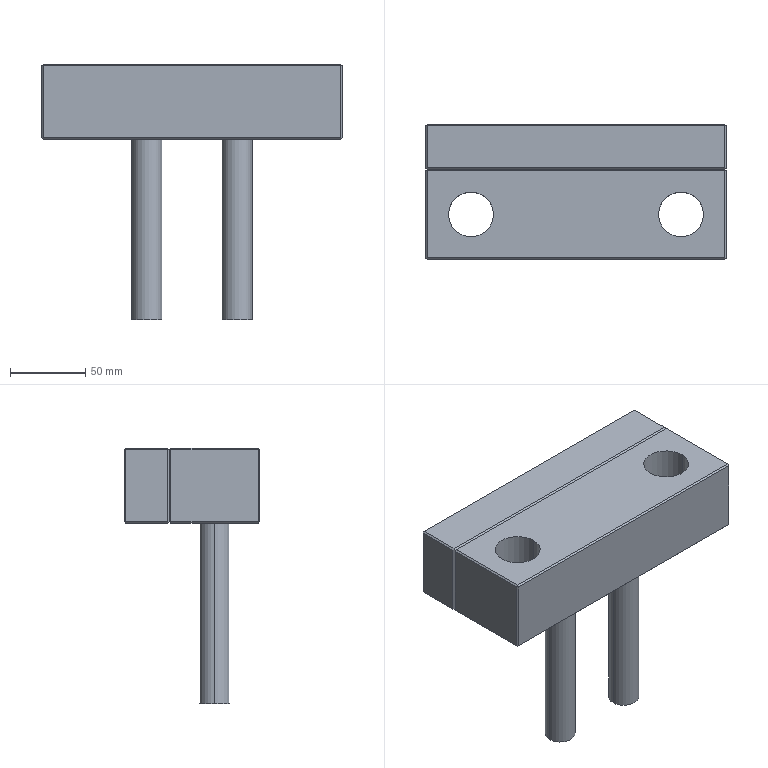Part | Creo | features CURVE 3, DATUM PLANE 3, PROTRUSION 3, CHAMFER 2, COORDINATE SYSTEM 1 | 1 solid | 44 faces | box 200 x 90 x 170 mm | volume 903544 mm3 | plane 36 | cylinder 8 | commonest cylinder face diameters 20 x4 30 x4
STEP:
#1=CARTESIAN_POINT('',(0.,0.,0.));
#2=DIRECTION('',(0.,0.,1.));
#3=DIRECTION('',(1.,0.,0.));
#4=AXIS2_PLACEMENT_3D('',#1,#2,#3);
#5=CARTESIAN_POINT('',(99.,29.,0.));
#6=VERTEX_POINT('',#5);
#7=CARTESIAN_POINT('',(99.,-29.,0.));
#8=VERTEX_POINT('',#7);
#9=CARTESIAN_POINT('',(99.,29.,0.));
#10=DIRECTION('',(0.,-1.,0.));
#11=VECTOR('',#10,58.);
#12=LINE('',#9,#11);
#13=EDGE_CURVE('',#6,#8,#12,.T.);
#14=ORIENTED_EDGE('',*,*,#13,.F.);
#15=CARTESIAN_POINT('',(-99.,29.,0.));
#16=VERTEX_POINT('',#15);
#17=CARTESIAN_POINT('',(-99.,29.,0.));
#18=DIRECTION('',(1.,0.,0.));
#19=VECTOR('',#18,198.);
#20=LINE('',#17,#19);
#21=EDGE_CURVE('',#16,#6,#20,.T.);
#22=ORIENTED_EDGE('',*,*,#21,.F.);
#23=CARTESIAN_POINT('',(-99.,-29.,0.));
#24=VERTEX_POINT('',#23);
#25=CARTESIAN_POINT('',(-99.,-29.,0.));
#26=DIRECTION('',(0.,1.,0.));
#27=VECTOR('',#26,58.);
#28=LINE('',#25,#27);
#29=EDGE_CURVE('',#24,#16,#28,.T.);
#30=ORIENTED_EDGE('',*,*,#29,.F.);
#31=CARTESIAN_POINT('',(99.,-29.,0.));
#32=DIRECTION('',(-1.,0.,0.));
#33=VECTOR('',#32,198.);
#34=LINE('',#31,#33);
#35=EDGE_CURVE('',#8,#24,#34,.T.);
#36=ORIENTED_EDGE('',*,*,#35,.F.);
#37=EDGE_LOOP('',(#14,#22,#30,#36));
#38=FACE_OUTER_BOUND('',#37,.F.);
#39=CARTESIAN_POINT('',(-55.,0.,0.));
#40=VERTEX_POINT('',#39);
#41=CARTESIAN_POINT('',(-85.,0.,0.));
#42=VERTEX_POINT('',#41);
#43=CARTESIAN_POINT('',(-70.,0.,0.));
#44=DIRECTION('',(0.,0.,-1.));
#45=DIRECTION('',(1.,0.,0.));
#46=AXIS2_PLACEMENT_3D('',#43,#44,#45);
#47=CIRCLE('',#46,15.);
#48=EDGE_CURVE('',#40,#42,#47,.T.);
#49=ORIENTED_EDGE('',*,*,#48,.T.);
#50=CARTESIAN_POINT('',(-70.,0.,0.));
#51=DIRECTION('',(0.,0.,-1.));
#52=DIRECTION('',(-1.,0.,0.));
#53=AXIS2_PLACEMENT_3D('',#50,#51,#52);
#54=CIRCLE('',#53,15.);
#55=EDGE_CURVE('',#42,#40,#54,.T.);
#56=ORIENTED_EDGE('',*,*,#55,.T.);
#57=EDGE_LOOP('',(#49,#56));
#58=FACE_BOUND('',#57,.F.);
#59=CARTESIAN_POINT('',(-40.,0.,0.));
#60=VERTEX_POINT('',#59);
#61=CARTESIAN_POINT('',(-20.,0.,0.));
#62=VERTEX_POINT('',#61);
#63=CARTESIAN_POINT('',(-30.,0.,0.));
#64=DIRECTION('',(0.,0.,-1.));
#65=DIRECTION('',(-1.,0.,0.));
#66=AXIS2_PLACEMENT_3D('',#63,#64,#65);
#67=CIRCLE('',#66,10.);
#68=EDGE_CURVE('',#60,#62,#67,.T.);
#69=ORIENTED_EDGE('',*,*,#68,.T.);
#70=CARTESIAN_POINT('',(-30.,0.,0.));
#71=DIRECTION('',(0.,0.,-1.));
#72=DIRECTION('',(1.,0.,0.));
#73=AXIS2_PLACEMENT_3D('',#70,#71,#72);
#74=CIRCLE('',#73,10.);
#75=EDGE_CURVE('',#62,#60,#74,.T.);
#76=ORIENTED_EDGE('',*,*,#75,.T.);
#77=EDGE_LOOP('',(#69,#76));
#78=FACE_BOUND('',#77,.F.);
#79=CARTESIAN_POINT('',(20.,0.,0.));
#80=VERTEX_POINT('',#79);
#81=CARTESIAN_POINT('',(40.,0.,0.));
#82=VERTEX_POINT('',#81);
#83=CARTESIAN_POINT('',(30.,0.,0.));
#84=DIRECTION('',(0.,0.,-1.));
#85=DIRECTION('',(-1.,0.,0.));
#86=AXIS2_PLACEMENT_3D('',#83,#84,#85);
#87=CIRCLE('',#86,10.);
#88=EDGE_CURVE('',#80,#82,#87,.T.);
#89=ORIENTED_EDGE('',*,*,#88,.T.);
#90=CARTESIAN_POINT('',(30.,0.,0.));
#91=DIRECTION('',(0.,0.,-1.));
#92=DIRECTION('',(1.,0.,0.));
#93=AXIS2_PLACEMENT_3D('',#90,#91,#92);
#94=CIRCLE('',#93,10.);
#95=EDGE_CURVE('',#82,#80,#94,.T.);
#96=ORIENTED_EDGE('',*,*,#95,.T.);
#97=EDGE_LOOP('',(#89,#96));
#98=FACE_BOUND('',#97,.F.);
#99=CARTESIAN_POINT('',(85.,0.,0.));
#100=VERTEX_POINT('',#99);
#101=CARTESIAN_POINT('',(55.,0.,0.));
#102=VERTEX_POINT('',#101);
#103=CARTESIAN_POINT('',(70.,0.,0.));
#104=DIRECTION('',(0.,0.,-1.));
#105=DIRECTION('',(1.,0.,0.));
#106=AXIS2_PLACEMENT_3D('',#103,#104,#105);
#107=CIRCLE('',#106,15.);
#108=EDGE_CURVE('',#100,#102,#107,.T.);
#109=ORIENTED_EDGE('',*,*,#108,.T.);
#110=CARTESIAN_POINT('',(70.,0.,0.));
#111=DIRECTION('',(0.,0.,-1.));
#112=DIRECTION('',(-1.,0.,0.));
#113=AXIS2_PLACEMENT_3D('',#110,#111,#112);
#114=CIRCLE('',#113,15.);
#115=EDGE_CURVE('',#102,#100,#114,.T.);
#116=ORIENTED_EDGE('',*,*,#115,.T.);
#117=EDGE_LOOP('',(#109,#116));
#118=FACE_BOUND('',#117,.F.);
#119=CARTESIAN_POINT('',(0.,0.,0.));
#120=DIRECTION('',(0.,0.,1.));
#121=DIRECTION('',(1.,0.,0.));
#122=AXIS2_PLACEMENT_3D('',#119,#120,#121);
#123=PLANE('',#122);
#124=ADVANCED_FACE('',(#38,#58,#78,#98,#118),#123,.F.);
#125=ORIENTED_EDGE('',*,*,#108,.F.);
#126=CARTESIAN_POINT('',(85.,0.,50.));
#127=VERTEX_POINT('',#126);
#128=CARTESIAN_POINT('',(85.,0.,0.));
#129=DIRECTION('',(0.,0.,1.));
#130=VECTOR('',#129,50.);
#131=LINE('',#128,#130);
#132=EDGE_CURVE('',#100,#127,#131,.T.);
#133=ORIENTED_EDGE('',*,*,#132,.T.);
#134=CARTESIAN_POINT('',(55.,0.,50.));
#135=VERTEX_POINT('',#134);
#136=CARTESIAN_POINT('',(70.,0.,50.));
#137=DIRECTION('',(0.,0.,-1.));
#138=DIRECTION('',(1.,0.,0.));
#139=AXIS2_PLACEMENT_3D('',#136,#137,#138);
#140=CIRCLE('',#139,15.);
#141=EDGE_CURVE('',#127,#135,#140,.T.);
#142=ORIENTED_EDGE('',*,*,#141,.T.);
#143=CARTESIAN_POINT('',(55.,0.,0.));
#144=DIRECTION('',(0.,0.,1.));
#145=VECTOR('',#144,50.);
#146=LINE('',#143,#145);
#147=EDGE_CURVE('',#102,#135,#146,.T.);
#148=ORIENTED_EDGE('',*,*,#147,.F.);
#149=EDGE_LOOP('',(#125,#133,#142,#148));
#150=FACE_OUTER_BOUND('',#149,.F.);
#151=CARTESIAN_POINT('',(70.,0.,0.));
#152=DIRECTION('',(0.,0.,1.));
#153=DIRECTION('',(1.,0.,0.));
#154=AXIS2_PLACEMENT_3D('',#151,#152,#153);
#155=CYLINDRICAL_SURFACE('',#154,15.);
#156=ADVANCED_FACE('',(#150),#155,.F.);
#157=ORIENTED_EDGE('',*,*,#115,.F.);
#158=ORIENTED_EDGE('',*,*,#147,.T.);
#159=CARTESIAN_POINT('',(70.,0.,50.));
#160=DIRECTION('',(0.,0.,-1.));
#161=DIRECTION('',(-1.,0.,0.));
#162=AXIS2_PLACEMENT_3D('',#159,#160,#161);
#163=CIRCLE('',#162,15.);
#164=EDGE_CURVE('',#135,#127,#163,.T.);
#165=ORIENTED_EDGE('',*,*,#164,.T.);
#166=ORIENTED_EDGE('',*,*,#132,.F.);
#167=EDGE_LOOP('',(#157,#158,#165,#166));
#168=FACE_OUTER_BOUND('',#167,.F.);
#169=CARTESIAN_POINT('',(70.,0.,0.));
#170=DIRECTION('',(0.,0.,1.));
#171=DIRECTION('',(1.,0.,0.));
#172=AXIS2_PLACEMENT_3D('',#169,#170,#171);
#173=CYLINDRICAL_SURFACE('',#172,15.);
#174=ADVANCED_FACE('',(#168),#173,.F.);
#175=CARTESIAN_POINT('',(99.,29.,50.));
#176=VERTEX_POINT('',#175);
#177=CARTESIAN_POINT('',(-99.,29.,50.));
#178=VERTEX_POINT('',#177);
#179=CARTESIAN_POINT('',(99.,29.,50.));
#180=DIRECTION('',(-1.,0.,0.));
#181=VECTOR('',#180,198.);
#182=LINE('',#179,#181);
#183=EDGE_CURVE('',#176,#178,#182,.T.);
#184=ORIENTED_EDGE('',*,*,#183,.F.);
#185=CARTESIAN_POINT('',(99.,-29.,50.));
#186=VERTEX_POINT('',#185);
#187=CARTESIAN_POINT('',(99.,-29.,50.));
#188=DIRECTION('',(0.,1.,0.));
#189=VECTOR('',#188,58.);
#190=LINE('',#187,#189);
#191=EDGE_CURVE('',#186,#176,#190,.T.);
#192=ORIENTED_EDGE('',*,*,#191,.F.);
#193=CARTESIAN_POINT('',(-99.,-29.,50.));
#194=VERTEX_POINT('',#193);
#195=CARTESIAN_POINT('',(-99.,-29.,50.));
#196=DIRECTION('',(1.,0.,0.));
#197=VECTOR('',#196,198.);
#198=LINE('',#195,#197);
#199=EDGE_CURVE('',#194,#186,#198,.T.);
#200=ORIENTED_EDGE('',*,*,#199,.F.);
#201=CARTESIAN_POINT('',(-99.,29.,50.));
#202=DIRECTION('',(0.,-1.,0.));
#203=VECTOR('',#202,58.);
#204=LINE('',#201,#203);
#205=EDGE_CURVE('',#178,#194,#204,.T.);
#206=ORIENTED_EDGE('',*,*,#205,.F.);
#207=EDGE_LOOP('',(#184,#192,#200,#206));
#208=FACE_OUTER_BOUND('',#207,.F.);
#209=CARTESIAN_POINT('',(-55.,0.,50.));
#210=VERTEX_POINT('',#209);
#211=CARTESIAN_POINT('',(-85.,0.,50.));
#212=VERTEX_POINT('',#211);
#213=CARTESIAN_POINT('',(-70.,0.,50.));
#214=DIRECTION('',(0.,0.,-1.));
#215=DIRECTION('',(1.,0.,0.));
#216=AXIS2_PLACEMENT_3D('',#213,#214,#215);
#217=CIRCLE('',#216,15.);
#218=EDGE_CURVE('',#210,#212,#217,.T.);
#219=ORIENTED_EDGE('',*,*,#218,.F.);
#220=CARTESIAN_POINT('',(-70.,0.,50.));
#221=DIRECTION('',(0.,0.,-1.));
#222=DIRECTION('',(-1.,0.,0.));
#223=AXIS2_PLACEMENT_3D('',#220,#221,#222);
#224=CIRCLE('',#223,15.);
#225=EDGE_CURVE('',#212,#210,#224,.T.);
#226=ORIENTED_EDGE('',*,*,#225,.F.);
#227=EDGE_LOOP('',(#219,#226));
#228=FACE_BOUND('',#227,.F.);
#229=ORIENTED_EDGE('',*,*,#141,.F.);
#230=ORIENTED_EDGE('',*,*,#164,.F.);
#231=EDGE_LOOP('',(#229,#230));
#232=FACE_BOUND('',#231,.F.);
#233=CARTESIAN_POINT('',(0.,0.,50.));
#234=DIRECTION('',(0.,0.,1.));
#235=DIRECTION('',(1.,0.,0.));
#236=AXIS2_PLACEMENT_3D('',#233,#234,#235);
#237=PLANE('',#236);
#238=ADVANCED_FACE('',(#208,#228,#232),#237,.T.);
#239=ORIENTED_EDGE('',*,*,#48,.F.);
#240=CARTESIAN_POINT('',(-55.,0.,0.));
#241=DIRECTION('',(0.,0.,1.));
#242=VECTOR('',#241,50.);
#243=LINE('',#240,#242);
#244=EDGE_CURVE('',#40,#210,#243,.T.);
#245=ORIENTED_EDGE('',*,*,#244,.T.);
#246=ORIENTED_EDGE('',*,*,#218,.T.);
#247=CARTESIAN_POINT('',(-85.,0.,0.));
#248=DIRECTION('',(0.,0.,1.));
#249=VECTOR('',#248,50.);
#250=LINE('',#247,#249);
#251=EDGE_CURVE('',#42,#212,#250,.T.);
#252=ORIENTED_EDGE('',*,*,#251,.F.);
#253=EDGE_LOOP('',(#239,#245,#246,#252));
#254=FACE_OUTER_BOUND('',#253,.F.);
#255=CARTESIAN_POINT('',(-70.,0.,0.));
#256=DIRECTION('',(0.,0.,1.));
#257=DIRECTION('',(1.,0.,0.));
#258=AXIS2_PLACEMENT_3D('',#255,#256,#257);
#259=CYLINDRICAL_SURFACE('',#258,15.);
#260=ADVANCED_FACE('',(#254),#259,.F.);
#261=ORIENTED_EDGE('',*,*,#55,.F.);
#262=ORIENTED_EDGE('',*,*,#251,.T.);
#263=ORIENTED_EDGE('',*,*,#225,.T.);
#264=ORIENTED_EDGE('',*,*,#244,.F.);
#265=EDGE_LOOP('',(#261,#262,#263,#264));
#266=FACE_OUTER_BOUND('',#265,.F.);
#267=CARTESIAN_POINT('',(-70.,0.,0.));
#268=DIRECTION('',(0.,0.,1.));
#269=DIRECTION('',(1.,0.,0.));
#270=AXIS2_PLACEMENT_3D('',#267,#268,#269);
#271=CYLINDRICAL_SURFACE('',#270,15.);
#272=ADVANCED_FACE('',(#266),#271,.F.);
#273=CARTESIAN_POINT('',(99.,30.,49.));
#274=VERTEX_POINT('',#273);
#275=CARTESIAN_POINT('',(-99.,30.,49.));
#276=VERTEX_POINT('',#275);
#277=CARTESIAN_POINT('',(99.,30.,49.));
#278=DIRECTION('',(-1.,0.,0.));
#279=VECTOR('',#278,198.);
#280=LINE('',#277,#279);
#281=EDGE_CURVE('',#274,#276,#280,.T.);
#282=ORIENTED_EDGE('',*,*,#281,.F.);
#283=CARTESIAN_POINT('',(99.5,29.5,49.5));
#284=VERTEX_POINT('',#283);
#285=CARTESIAN_POINT('',(99.,30.,49.));
#286=DIRECTION('',(0.5774,-0.5774,0.5774));
#287=VECTOR('',#286,0.866);
#288=LINE('',#285,#287);
#289=EDGE_CURVE('',#274,#284,#288,.T.);
#290=ORIENTED_EDGE('',*,*,#289,.T.);
#291=CARTESIAN_POINT('',(99.,29.,50.));
#292=DIRECTION('',(0.5774,0.5774,-0.5774));
#293=VECTOR('',#292,0.866);
#294=LINE('',#291,#293);
#295=EDGE_CURVE('',#176,#284,#294,.T.);
#296=ORIENTED_EDGE('',*,*,#295,.F.);
#297=ORIENTED_EDGE('',*,*,#183,.T.);
#298=CARTESIAN_POINT('',(-99.5,29.5,49.5));
#299=VERTEX_POINT('',#298);
#300=CARTESIAN_POINT('',(-99.,29.,50.));
#301=DIRECTION('',(-0.5774,0.5774,-0.5774));
#302=VECTOR('',#301,0.866);
#303=LINE('',#300,#302);
#304=EDGE_CURVE('',#178,#299,#303,.T.);
#305=ORIENTED_EDGE('',*,*,#304,.T.);
#306=CARTESIAN_POINT('',(-99.5,29.5,49.5));
#307=DIRECTION('',(0.5774,0.5774,-0.5774));
#308=VECTOR('',#307,0.866);
#309=LINE('',#306,#308);
#310=EDGE_CURVE('',#299,#276,#309,.T.);
#311=ORIENTED_EDGE('',*,*,#310,.T.);
#312=EDGE_LOOP('',(#282,#290,#296,#297,#305,#311));
#313=FACE_OUTER_BOUND('',#312,.F.);
#314=CARTESIAN_POINT('',(0.,29.5,49.5));
#315=DIRECTION('',(0.,0.7071,0.7071));
#316=DIRECTION('',(0.,0.7071,-0.7071));
#317=AXIS2_PLACEMENT_3D('',#314,#315,#316);
#318=PLANE('',#317);
#319=ADVANCED_FACE('',(#313),#318,.T.);
#320=CARTESIAN_POINT('',(-99.5,30.5,49.5));
#321=VERTEX_POINT('',#320);
#322=CARTESIAN_POINT('',(-99.,31.,50.));
#323=VERTEX_POINT('',#322);
#324=CARTESIAN_POINT('',(-99.5,30.5,49.5));
#325=DIRECTION('',(0.5774,0.5774,0.5774));
#326=VECTOR('',#325,0.866);
#327=LINE('',#324,#326);
#328=EDGE_CURVE('',#321,#323,#327,.T.);
#329=ORIENTED_EDGE('',*,*,#328,.T.);
#330=CARTESIAN_POINT('',(99.,31.,50.));
#331=VERTEX_POINT('',#330);
#332=CARTESIAN_POINT('',(99.,31.,50.));
#333=DIRECTION('',(-1.,0.,0.));
#334=VECTOR('',#333,198.);
#335=LINE('',#332,#334);
#336=EDGE_CURVE('',#331,#323,#335,.T.);
#337=ORIENTED_EDGE('',*,*,#336,.F.);
#338=CARTESIAN_POINT('',(99.5,30.5,49.5));
#339=VERTEX_POINT('',#338);
#340=CARTESIAN_POINT('',(99.,31.,50.));
#341=DIRECTION('',(0.5774,-0.5774,-0.5774));
#342=VECTOR('',#341,0.866);
#343=LINE('',#340,#342);
#344=EDGE_CURVE('',#331,#339,#343,.T.);
#345=ORIENTED_EDGE('',*,*,#344,.T.);
#346=CARTESIAN_POINT('',(99.5,30.5,49.5));
#347=DIRECTION('',(-0.5774,-0.5774,-0.5774));
#348=VECTOR('',#347,0.866);
#349=LINE('',#346,#348);
#350=EDGE_CURVE('',#339,#274,#349,.T.);
#351=ORIENTED_EDGE('',*,*,#350,.T.);
#352=ORIENTED_EDGE('',*,*,#281,.T.);
#353=CARTESIAN_POINT('',(-99.5,30.5,49.5));
#354=DIRECTION('',(0.5774,-0.5774,-0.5774));
#355=VECTOR('',#354,0.866);
#356=LINE('',#353,#355);
#357=EDGE_CURVE('',#321,#276,#356,.T.);
#358=ORIENTED_EDGE('',*,*,#357,.F.);
#359=EDGE_LOOP('',(#329,#337,#345,#351,#352,#358));
#360=FACE_OUTER_BOUND('',#359,.F.);
#361=CARTESIAN_POINT('',(0.,30.5,49.5));
#362=DIRECTION('',(0.,-0.7071,0.7071));
#363=DIRECTION('',(0.,0.7071,0.7071));
#364=AXIS2_PLACEMENT_3D('',#361,#362,#363);
#365=PLANE('',#364);
#366=ADVANCED_FACE('',(#360),#365,.T.);
#367=CARTESIAN_POINT('',(-99.5,59.5,49.5));
#368=VERTEX_POINT('',#367);
#369=CARTESIAN_POINT('',(-100.,59.,49.));
#370=VERTEX_POINT('',#369);
#371=CARTESIAN_POINT('',(-99.5,59.5,49.5));
#372=DIRECTION('',(-0.5774,-0.5774,-0.5774));
#373=VECTOR('',#372,0.866);
#374=LINE('',#371,#373);
#375=EDGE_CURVE('',#368,#370,#374,.T.);
#376=ORIENTED_EDGE('',*,*,#375,.F.);
#377=CARTESIAN_POINT('',(-99.,59.,50.));
#378=VERTEX_POINT('',#377);
#379=CARTESIAN_POINT('',(-99.,59.,50.));
#380=DIRECTION('',(-0.5774,0.5774,-0.5774));
#381=VECTOR('',#380,0.866);
#382=LINE('',#379,#381);
#383=EDGE_CURVE('',#378,#368,#382,.T.);
#384=ORIENTED_EDGE('',*,*,#383,.F.);
#385=CARTESIAN_POINT('',(-99.,31.,50.));
#386=DIRECTION('',(0.,1.,0.));
#387=VECTOR('',#386,28.);
#388=LINE('',#385,#387);
#389=EDGE_CURVE('',#323,#378,#388,.T.);
#390=ORIENTED_EDGE('',*,*,#389,.F.);
#391=ORIENTED_EDGE('',*,*,#328,.F.);
#392=CARTESIAN_POINT('',(-100.,31.,49.));
#393=VERTEX_POINT('',#392);
#394=CARTESIAN_POINT('',(-100.,31.,49.));
#395=DIRECTION('',(0.5774,-0.5774,0.5774));
#396=VECTOR('',#395,0.866);
#397=LINE('',#394,#396);
#398=EDGE_CURVE('',#393,#321,#397,.T.);
#399=ORIENTED_EDGE('',*,*,#398,.F.);
#400=CARTESIAN_POINT('',(-100.,31.,49.));
#401=DIRECTION('',(0.,1.,0.));
#402=VECTOR('',#401,28.);
#403=LINE('',#400,#402);
#404=EDGE_CURVE('',#393,#370,#403,.T.);
#405=ORIENTED_EDGE('',*,*,#404,.T.);
#406=EDGE_LOOP('',(#376,#384,#390,#391,#399,#405));
#407=FACE_OUTER_BOUND('',#406,.F.);
#408=CARTESIAN_POINT('',(-100.,30.,49.));
#409=DIRECTION('',(-0.7071,0.,0.7071));
#410=DIRECTION('',(0.7071,0.,0.7071));
#411=AXIS2_PLACEMENT_3D('',#408,#409,#410);
#412=PLANE('',#411);
#413=ADVANCED_FACE('',(#407),#412,.T.);
#414=ORIENTED_EDGE('',*,*,#375,.T.);
#415=CARTESIAN_POINT('',(-100.,59.,1.));
#416=VERTEX_POINT('',#415);
#417=CARTESIAN_POINT('',(-100.,59.,1.));
#418=DIRECTION('',(0.,0.,1.));
#419=VECTOR('',#418,48.);
#420=LINE('',#417,#419);
#421=EDGE_CURVE('',#416,#370,#420,.T.);
#422=ORIENTED_EDGE('',*,*,#421,.F.);
#423=CARTESIAN_POINT('',(-99.5,59.5,0.5));
#424=VERTEX_POINT('',#423);
#425=CARTESIAN_POINT('',(-100.,59.,1.));
#426=DIRECTION('',(0.5774,0.5774,-0.5774));
#427=VECTOR('',#426,0.866);
#428=LINE('',#425,#427);
#429=EDGE_CURVE('',#416,#424,#428,.T.);
#430=ORIENTED_EDGE('',*,*,#429,.T.);
#431=CARTESIAN_POINT('',(-99.,60.,1.));
#432=VERTEX_POINT('',#431);
#433=CARTESIAN_POINT('',(-99.5,59.5,0.5));
#434=DIRECTION('',(0.5774,0.5774,0.5774));
#435=VECTOR('',#434,0.866);
#436=LINE('',#433,#435);
#437=EDGE_CURVE('',#424,#432,#436,.T.);
#438=ORIENTED_EDGE('',*,*,#437,.T.);
#439=CARTESIAN_POINT('',(-99.,60.,49.));
#440=VERTEX_POINT('',#439);
#441=CARTESIAN_POINT('',(-99.,60.,1.));
#442=DIRECTION('',(0.,0.,1.));
#443=VECTOR('',#442,48.);
#444=LINE('',#441,#443);
#445=EDGE_CURVE('',#432,#440,#444,.T.);
#446=ORIENTED_EDGE('',*,*,#445,.T.);
#447=CARTESIAN_POINT('',(-99.5,59.5,49.5));
#448=DIRECTION('',(0.5774,0.5774,-0.5774));
#449=VECTOR('',#448,0.866);
#450=LINE('',#447,#449);
#451=EDGE_CURVE('',#368,#440,#450,.T.);
#452=ORIENTED_EDGE('',*,*,#451,.F.);
#453=EDGE_LOOP('',(#414,#422,#430,#438,#446,#452));
#454=FACE_OUTER_BOUND('',#453,.F.);
#455=CARTESIAN_POINT('',(-99.5,59.5,25.));
#456=DIRECTION('',(-0.7071,0.7071,0.));
#457=DIRECTION('',(-0.7071,-0.7071,0.));
#458=AXIS2_PLACEMENT_3D('',#455,#456,#457);
#459=PLANE('',#458);
#460=ADVANCED_FACE('',(#454),#459,.T.);
#461=ORIENTED_EDGE('',*,*,#421,.T.);
#462=ORIENTED_EDGE('',*,*,#404,.F.);
#463=CARTESIAN_POINT('',(-100.,31.,1.));
#464=VERTEX_POINT('',#463);
#465=CARTESIAN_POINT('',(-100.,31.,49.));
#466=DIRECTION('',(0.,0.,-1.));
#467=VECTOR('',#466,48.);
#468=LINE('',#465,#467);
#469=EDGE_CURVE('',#393,#464,#468,.T.);
#470=ORIENTED_EDGE('',*,*,#469,.T.);
#471=CARTESIAN_POINT('',(-100.,31.,1.));
#472=DIRECTION('',(0.,1.,0.));
#473=VECTOR('',#472,28.);
#474=LINE('',#471,#473);
#475=EDGE_CURVE('',#464,#416,#474,.T.);
#476=ORIENTED_EDGE('',*,*,#475,.T.);
#477=EDGE_LOOP('',(#461,#462,#470,#476));
#478=FACE_OUTER_BOUND('',#477,.F.);
#479=CARTESIAN_POINT('',(-100.,30.,1.));
#480=DIRECTION('',(-1.,0.,0.));
#481=DIRECTION('',(0.,0.,1.));
#482=AXIS2_PLACEMENT_3D('',#479,#480,#481);
#483=PLANE('',#482);
#484=ADVANCED_FACE('',(#478),#483,.T.);
#485=ORIENTED_EDGE('',*,*,#398,.T.);
#486=ORIENTED_EDGE('',*,*,#357,.T.);
#487=CARTESIAN_POINT('',(-99.,30.,1.));
#488=VERTEX_POINT('',#487);
#489=CARTESIAN_POINT('',(-99.,30.,49.));
#490=DIRECTION('',(0.,0.,-1.));
#491=VECTOR('',#490,48.);
#492=LINE('',#489,#491);
#493=EDGE_CURVE('',#276,#488,#492,.T.);
#494=ORIENTED_EDGE('',*,*,#493,.T.);
#495=CARTESIAN_POINT('',(-99.5,30.5,0.5));
#496=VERTEX_POINT('',#495);
#497=CARTESIAN_POINT('',(-99.5,30.5,0.5));
#498=DIRECTION('',(0.5774,-0.5774,0.5774));
#499=VECTOR('',#498,0.866);
#500=LINE('',#497,#499);
#501=EDGE_CURVE('',#496,#488,#500,.T.);
#502=ORIENTED_EDGE('',*,*,#501,.F.);
#503=CARTESIAN_POINT('',(-99.5,30.5,0.5));
#504=DIRECTION('',(-0.5774,0.5774,0.5774));
#505=VECTOR('',#504,0.866);
#506=LINE('',#503,#505);
#507=EDGE_CURVE('',#496,#464,#506,.T.);
#508=ORIENTED_EDGE('',*,*,#507,.T.);
#509=ORIENTED_EDGE('',*,*,#469,.F.);
#510=EDGE_LOOP('',(#485,#486,#494,#502,#508,#509));
#511=FACE_OUTER_BOUND('',#510,.F.);
#512=CARTESIAN_POINT('',(-99.5,30.5,25.));
#513=DIRECTION('',(-0.7071,-0.7071,0.));
#514=DIRECTION('',(-0.7071,0.7071,0.));
#515=AXIS2_PLACEMENT_3D('',#512,#513,#514);
#516=PLANE('',#515);
#517=ADVANCED_FACE('',(#511),#516,.T.);
#518=ORIENTED_EDGE('',*,*,#493,.F.);
#519=ORIENTED_EDGE('',*,*,#310,.F.);
#520=CARTESIAN_POINT('',(-100.,29.,49.));
#521=VERTEX_POINT('',#520);
#522=CARTESIAN_POINT('',(-100.,29.,49.));
#523=DIRECTION('',(0.5774,0.5774,0.5774));
#524=VECTOR('',#523,0.866);
#525=LINE('',#522,#524);
#526=EDGE_CURVE('',#521,#299,#525,.T.);
#527=ORIENTED_EDGE('',*,*,#526,.F.);
#528=CARTESIAN_POINT('',(-100.,29.,1.));
#529=VERTEX_POINT('',#528);
#530=CARTESIAN_POINT('',(-100.,29.,49.));
#531=DIRECTION('',(0.,0.,-1.));
#532=VECTOR('',#531,48.);
#533=LINE('',#530,#532);
#534=EDGE_CURVE('',#521,#529,#533,.T.);
#535=ORIENTED_EDGE('',*,*,#534,.T.);
#536=CARTESIAN_POINT('',(-99.5,29.5,0.5));
#537=VERTEX_POINT('',#536);
#538=CARTESIAN_POINT('',(-100.,29.,1.));
#539=DIRECTION('',(0.5774,0.5774,-0.5774));
#540=VECTOR('',#539,0.866);
#541=LINE('',#538,#540);
#542=EDGE_CURVE('',#529,#537,#541,.T.);
#543=ORIENTED_EDGE('',*,*,#542,.T.);
#544=CARTESIAN_POINT('',(-99.,30.,1.));
#545=DIRECTION('',(-0.5774,-0.5774,-0.5774));
#546=VECTOR('',#545,0.866);
#547=LINE('',#544,#546);
#548=EDGE_CURVE('',#488,#537,#547,.T.);
#549=ORIENTED_EDGE('',*,*,#548,.F.);
#550=EDGE_LOOP('',(#518,#519,#527,#535,#543,#549));
#551=FACE_OUTER_BOUND('',#550,.F.);
#552=CARTESIAN_POINT('',(-99.5,29.5,25.));
#553=DIRECTION('',(-0.7071,0.7071,0.));
#554=DIRECTION('',(0.7071,0.7071,0.));
#555=AXIS2_PLACEMENT_3D('',#552,#553,#554);
#556=PLANE('',#555);
#557=ADVANCED_FACE('',(#551),#556,.T.);
#558=CARTESIAN_POINT('',(-100.,-29.,49.));
#559=VERTEX_POINT('',#558);
#560=CARTESIAN_POINT('',(-100.,29.,49.));
#561=DIRECTION('',(0.,-1.,0.));
#562=VECTOR('',#561,58.);
#563=LINE('',#560,#562);
#564=EDGE_CURVE('',#521,#559,#563,.T.);
#565=ORIENTED_EDGE('',*,*,#564,.F.);
#566=ORIENTED_EDGE('',*,*,#526,.T.);
#567=ORIENTED_EDGE('',*,*,#304,.F.);
#568=ORIENTED_EDGE('',*,*,#205,.T.);
#569=CARTESIAN_POINT('',(-99.5,-29.5,49.5));
#570=VERTEX_POINT('',#569);
#571=CARTESIAN_POINT('',(-99.,-29.,50.));
#572=DIRECTION('',(-0.5774,-0.5774,-0.5774));
#573=VECTOR('',#572,0.866);
#574=LINE('',#571,#573);
#575=EDGE_CURVE('',#194,#570,#574,.T.);
#576=ORIENTED_EDGE('',*,*,#575,.T.);
#577=CARTESIAN_POINT('',(-99.5,-29.5,49.5));
#578=DIRECTION('',(-0.5774,0.5774,-0.5774));
#579=VECTOR('',#578,0.866);
#580=LINE('',#577,#579);
#581=EDGE_CURVE('',#570,#559,#580,.T.);
#582=ORIENTED_EDGE('',*,*,#581,.T.);
#583=EDGE_LOOP('',(#565,#566,#567,#568,#576,#582));
#584=FACE_OUTER_BOUND('',#583,.F.);
#585=CARTESIAN_POINT('',(-99.5,0.,49.5));
#586=DIRECTION('',(-0.7071,0.,0.7071));
#587=DIRECTION('',(-0.7071,0.,-0.7071));
#588=AXIS2_PLACEMENT_3D('',#585,#586,#587);
#589=PLANE('',#588);
#590=ADVANCED_FACE('',(#584),#589,.T.);
#591=ORIENTED_EDGE('',*,*,#564,.T.);
#592=CARTESIAN_POINT('',(-100.,-29.,1.));
#593=VERTEX_POINT('',#592);
#594=CARTESIAN_POINT('',(-100.,-29.,49.));
#595=DIRECTION('',(0.,0.,-1.));
#596=VECTOR('',#595,48.);
#597=LINE('',#594,#596);
#598=EDGE_CURVE('',#559,#593,#597,.T.);
#599=ORIENTED_EDGE('',*,*,#598,.T.);
#600=CARTESIAN_POINT('',(-100.,-29.,1.));
#601=DIRECTION('',(0.,1.,0.));
#602=VECTOR('',#601,58.);
#603=LINE('',#600,#602);
#604=EDGE_CURVE('',#593,#529,#603,.T.);
#605=ORIENTED_EDGE('',*,*,#604,.T.);
#606=ORIENTED_EDGE('',*,*,#534,.F.);
#607=EDGE_LOOP('',(#591,#599,#605,#606));
#608=FACE_OUTER_BOUND('',#607,.F.);
#609=CARTESIAN_POINT('',(-100.,30.,0.));
#610=DIRECTION('',(-1.,0.,0.));
#611=DIRECTION('',(0.,-1.,0.));
#612=AXIS2_PLACEMENT_3D('',#609,#610,#611);
#613=PLANE('',#612);
#614=ADVANCED_FACE('',(#608),#613,.T.);
#615=CARTESIAN_POINT('',(-99.,-30.,49.));
#616=VERTEX_POINT('',#615);
#617=CARTESIAN_POINT('',(-99.,-30.,1.));
#618=VERTEX_POINT('',#617);
#619=CARTESIAN_POINT('',(-99.,-30.,49.));
#620=DIRECTION('',(0.,0.,-1.));
#621=VECTOR('',#620,48.);
#622=LINE('',#619,#621);
#623=EDGE_CURVE('',#616,#618,#622,.T.);
#624=ORIENTED_EDGE('',*,*,#623,.T.);
#625=CARTESIAN_POINT('',(-99.5,-29.5,0.5));
#626=VERTEX_POINT('',#625);
#627=CARTESIAN_POINT('',(-99.,-30.,1.));
#628=DIRECTION('',(-0.5774,0.5774,-0.5774));
#629=VECTOR('',#628,0.866);
#630=LINE('',#627,#629);
#631=EDGE_CURVE('',#618,#626,#630,.T.);
#632=ORIENTED_EDGE('',*,*,#631,.T.);
#633=CARTESIAN_POINT('',(-100.,-29.,1.));
#634=DIRECTION('',(0.5774,-0.5774,-0.5774));
#635=VECTOR('',#634,0.866);
#636=LINE('',#633,#635);
#637=EDGE_CURVE('',#593,#626,#636,.T.);
#638=ORIENTED_EDGE('',*,*,#637,.F.);
#639=ORIENTED_EDGE('',*,*,#598,.F.);
#640=ORIENTED_EDGE('',*,*,#581,.F.);
#641=CARTESIAN_POINT('',(-99.,-30.,49.));
#642=DIRECTION('',(-0.5774,0.5774,0.5774));
#643=VECTOR('',#642,0.866);
#644=LINE('',#641,#643);
#645=EDGE_CURVE('',#616,#570,#644,.T.);
#646=ORIENTED_EDGE('',*,*,#645,.F.);
#647=EDGE_LOOP('',(#624,#632,#638,#639,#640,#646));
#648=FACE_OUTER_BOUND('',#647,.F.);
#649=CARTESIAN_POINT('',(-99.5,-29.5,25.));
#650=DIRECTION('',(-0.7071,-0.7071,0.));
#651=DIRECTION('',(-0.7071,0.7071,0.));
#652=AXIS2_PLACEMENT_3D('',#649,#650,#651);
#653=PLANE('',#652);
#654=ADVANCED_FACE('',(#648),#653,.T.);
#655=CARTESIAN_POINT('',(99.,-30.,49.));
#656=VERTEX_POINT('',#655);
#657=CARTESIAN_POINT('',(-99.,-30.,49.));
#658=DIRECTION('',(1.,0.,0.));
#659=VECTOR('',#658,198.);
#660=LINE('',#657,#659);
#661=EDGE_CURVE('',#616,#656,#660,.T.);
#662=ORIENTED_EDGE('',*,*,#661,.T.);
#663=CARTESIAN_POINT('',(99.,-30.,1.));
#664=VERTEX_POINT('',#663);
#665=CARTESIAN_POINT('',(99.,-30.,49.));
#666=DIRECTION('',(0.,0.,-1.));
#667=VECTOR('',#666,48.);
#668=LINE('',#665,#667);
#669=EDGE_CURVE('',#656,#664,#668,.T.);
#670=ORIENTED_EDGE('',*,*,#669,.T.);
#671=CARTESIAN_POINT('',(99.,-30.,1.));
#672=DIRECTION('',(-1.,0.,0.));
#673=VECTOR('',#672,198.);
#674=LINE('',#671,#673);
#675=EDGE_CURVE('',#664,#618,#674,.T.);
#676=ORIENTED_EDGE('',*,*,#675,.T.);
#677=ORIENTED_EDGE('',*,*,#623,.F.);
#678=EDGE_LOOP('',(#662,#670,#676,#677));
#679=FACE_OUTER_BOUND('',#678,.F.);
#680=CARTESIAN_POINT('',(-100.,-30.,0.));
#681=DIRECTION('',(0.,-1.,0.));
#682=DIRECTION('',(1.,0.,0.));
#683=AXIS2_PLACEMENT_3D('',#680,#681,#682);
#684=PLANE('',#683);
#685=ADVANCED_FACE('',(#679),#684,.T.);
#686=ORIENTED_EDGE('',*,*,#199,.T.);
#687=CARTESIAN_POINT('',(99.5,-29.5,49.5));
#688=VERTEX_POINT('',#687);
#689=CARTESIAN_POINT('',(99.5,-29.5,49.5));
#690=DIRECTION('',(-0.5774,0.5774,0.5774));
#691=VECTOR('',#690,0.866);
#692=LINE('',#689,#691);
#693=EDGE_CURVE('',#688,#186,#692,.T.);
#694=ORIENTED_EDGE('',*,*,#693,.F.);
#695=CARTESIAN_POINT('',(99.,-30.,49.));
#696=DIRECTION('',(0.5774,0.5774,0.5774));
#697=VECTOR('',#696,0.866);
#698=LINE('',#695,#697);
#699=EDGE_CURVE('',#656,#688,#698,.T.);
#700=ORIENTED_EDGE('',*,*,#699,.F.);
#701=ORIENTED_EDGE('',*,*,#661,.F.);
#702=ORIENTED_EDGE('',*,*,#645,.T.);
#703=ORIENTED_EDGE('',*,*,#575,.F.);
#704=EDGE_LOOP('',(#686,#694,#700,#701,#702,#703));
#705=FACE_OUTER_BOUND('',#704,.F.);
#706=CARTESIAN_POINT('',(0.,-29.5,49.5));
#707=DIRECTION('',(0.,-0.7071,0.7071));
#708=DIRECTION('',(0.,-0.7071,-0.7071));
#709=AXIS2_PLACEMENT_3D('',#706,#707,#708);
#710=PLANE('',#709);
#711=ADVANCED_FACE('',(#705),#710,.T.);
#712=CARTESIAN_POINT('',(100.,-29.,49.));
#713=VERTEX_POINT('',#712);
#714=CARTESIAN_POINT('',(100.,29.,49.));
#715=VERTEX_POINT('',#714);
#716=CARTESIAN_POINT('',(100.,-29.,49.));
#717=DIRECTION('',(0.,1.,0.));
#718=VECTOR('',#717,58.);
#719=LINE('',#716,#718);
#720=EDGE_CURVE('',#713,#715,#719,.T.);
#721=ORIENTED_EDGE('',*,*,#720,.F.);
#722=CARTESIAN_POINT('',(100.,-29.,49.));
#723=DIRECTION('',(-0.5774,-0.5774,0.5774));
#724=VECTOR('',#723,0.866);
#725=LINE('',#722,#724);
#726=EDGE_CURVE('',#713,#688,#725,.T.);
#727=ORIENTED_EDGE('',*,*,#726,.T.);
#728=ORIENTED_EDGE('',*,*,#693,.T.);
#729=ORIENTED_EDGE('',*,*,#191,.T.);
#730=ORIENTED_EDGE('',*,*,#295,.T.);
#731=CARTESIAN_POINT('',(99.5,29.5,49.5));
#732=DIRECTION('',(0.5774,-0.5774,-0.5774));
#733=VECTOR('',#732,0.866);
#734=LINE('',#731,#733);
#735=EDGE_CURVE('',#284,#715,#734,.T.);
#736=ORIENTED_EDGE('',*,*,#735,.T.);
#737=EDGE_LOOP('',(#721,#727,#728,#729,#730,#736));
#738=FACE_OUTER_BOUND('',#737,.F.);
#739=CARTESIAN_POINT('',(99.5,0.,49.5));
#740=DIRECTION('',(0.7071,0.,0.7071));
#741=DIRECTION('',(0.7071,0.,-0.7071));
#742=AXIS2_PLACEMENT_3D('',#739,#740,#741);
#743=PLANE('',#742);
#744=ADVANCED_FACE('',(#738),#743,.T.);
#745=CARTESIAN_POINT('',(100.,29.,1.));
#746=VERTEX_POINT('',#745);
#747=CARTESIAN_POINT('',(100.,-29.,1.));
#748=VERTEX_POINT('',#747);
#749=CARTESIAN_POINT('',(100.,29.,1.));
#750=DIRECTION('',(0.,-1.,0.));
#751=VECTOR('',#750,58.);
#752=LINE('',#749,#751);
#753=EDGE_CURVE('',#746,#748,#752,.T.);
#754=ORIENTED_EDGE('',*,*,#753,.T.);
#755=CARTESIAN_POINT('',(100.,-29.,49.));
#756=DIRECTION('',(0.,0.,-1.));
#757=VECTOR('',#756,48.);
#758=LINE('',#755,#757);
#759=EDGE_CURVE('',#713,#748,#758,.T.);
#760=ORIENTED_EDGE('',*,*,#759,.F.);
#761=ORIENTED_EDGE('',*,*,#720,.T.);
#762=CARTESIAN_POINT('',(100.,29.,49.));
#763=DIRECTION('',(0.,0.,-1.));
#764=VECTOR('',#763,48.);
#765=LINE('',#762,#764);
#766=EDGE_CURVE('',#715,#746,#765,.T.);
#767=ORIENTED_EDGE('',*,*,#766,.T.);
#768=EDGE_LOOP('',(#754,#760,#761,#767));
#769=FACE_OUTER_BOUND('',#768,.F.);
#770=CARTESIAN_POINT('',(100.,-30.,0.));
#771=DIRECTION('',(1.,0.,0.));
#772=DIRECTION('',(0.,1.,0.));
#773=AXIS2_PLACEMENT_3D('',#770,#771,#772);
#774=PLANE('',#773);
#775=ADVANCED_FACE('',(#769),#774,.T.);
#776=ORIENTED_EDGE('',*,*,#753,.F.);
#777=CARTESIAN_POINT('',(99.5,29.5,0.5));
#778=VERTEX_POINT('',#777);
#779=CARTESIAN_POINT('',(100.,29.,1.));
#780=DIRECTION('',(-0.5774,0.5774,-0.5774));
#781=VECTOR('',#780,0.866);
#782=LINE('',#779,#781);
#783=EDGE_CURVE('',#746,#778,#782,.T.);
#784=ORIENTED_EDGE('',*,*,#783,.T.);
#785=CARTESIAN_POINT('',(99.5,29.5,0.5));
#786=DIRECTION('',(-0.5774,-0.5774,-0.5774));
#787=VECTOR('',#786,0.866);
#788=LINE('',#785,#787);
#789=EDGE_CURVE('',#778,#6,#788,.T.);
#790=ORIENTED_EDGE('',*,*,#789,.T.);
#791=ORIENTED_EDGE('',*,*,#13,.T.);
#792=CARTESIAN_POINT('',(99.5,-29.5,0.5));
#793=VERTEX_POINT('',#792);
#794=CARTESIAN_POINT('',(99.,-29.,0.));
#795=DIRECTION('',(0.5774,-0.5774,0.5774));
#796=VECTOR('',#795,0.866);
#797=LINE('',#794,#796);
#798=EDGE_CURVE('',#8,#793,#797,.T.);
#799=ORIENTED_EDGE('',*,*,#798,.T.);
#800=CARTESIAN_POINT('',(99.5,-29.5,0.5));
#801=DIRECTION('',(0.5774,0.5774,0.5774));
#802=VECTOR('',#801,0.866);
#803=LINE('',#800,#802);
#804=EDGE_CURVE('',#793,#748,#803,.T.);
#805=ORIENTED_EDGE('',*,*,#804,.T.);
#806=EDGE_LOOP('',(#776,#784,#790,#791,#799,#805));
#807=FACE_OUTER_BOUND('',#806,.F.);
#808=CARTESIAN_POINT('',(99.5,0.,0.5));
#809=DIRECTION('',(0.7071,0.,-0.7071));
#810=DIRECTION('',(0.7071,0.,0.7071));
#811=AXIS2_PLACEMENT_3D('',#808,#809,#810);
#812=PLANE('',#811);
#813=ADVANCED_FACE('',(#807),#812,.T.);
#814=CARTESIAN_POINT('',(99.,30.,1.));
#815=VERTEX_POINT('',#814);
#816=CARTESIAN_POINT('',(99.,30.,1.));
#817=DIRECTION('',(0.,0.,1.));
#818=VECTOR('',#817,48.);
#819=LINE('',#816,#818);
#820=EDGE_CURVE('',#815,#274,#819,.T.);
#821=ORIENTED_EDGE('',*,*,#820,.F.);
#822=CARTESIAN_POINT('',(99.,30.,1.));
#823=DIRECTION('',(0.5774,-0.5774,-0.5774));
#824=VECTOR('',#823,0.866);
#825=LINE('',#822,#824);
#826=EDGE_CURVE('',#815,#778,#825,.T.);
#827=ORIENTED_EDGE('',*,*,#826,.T.);
#828=ORIENTED_EDGE('',*,*,#783,.F.);
#829=ORIENTED_EDGE('',*,*,#766,.F.);
#830=ORIENTED_EDGE('',*,*,#735,.F.);
#831=ORIENTED_EDGE('',*,*,#289,.F.);
#832=EDGE_LOOP('',(#821,#827,#828,#829,#830,#831));
#833=FACE_OUTER_BOUND('',#832,.F.);
#834=CARTESIAN_POINT('',(99.5,29.5,25.));
#835=DIRECTION('',(0.7071,0.7071,0.));
#836=DIRECTION('',(0.7071,-0.7071,0.));
#837=AXIS2_PLACEMENT_3D('',#834,#835,#836);
#838=PLANE('',#837);
#839=ADVANCED_FACE('',(#833),#838,.T.);
#840=CARTESIAN_POINT('',(100.,31.,49.));
#841=VERTEX_POINT('',#840);
#842=CARTESIAN_POINT('',(99.5,30.5,49.5));
#843=DIRECTION('',(0.5774,0.5774,-0.5774));
#844=VECTOR('',#843,0.866);
#845=LINE('',#842,#844);
#846=EDGE_CURVE('',#339,#841,#845,.T.);
#847=ORIENTED_EDGE('',*,*,#846,.T.);
#848=CARTESIAN_POINT('',(100.,31.,1.));
#849=VERTEX_POINT('',#848);
#850=CARTESIAN_POINT('',(100.,31.,1.));
#851=DIRECTION('',(0.,0.,1.));
#852=VECTOR('',#851,48.);
#853=LINE('',#850,#852);
#854=EDGE_CURVE('',#849,#841,#853,.T.);
#855=ORIENTED_EDGE('',*,*,#854,.F.);
#856=CARTESIAN_POINT('',(99.5,30.5,0.5));
#857=VERTEX_POINT('',#856);
#858=CARTESIAN_POINT('',(100.,31.,1.));
#859=DIRECTION('',(-0.5774,-0.5774,-0.5774));
#860=VECTOR('',#859,0.866);
#861=LINE('',#858,#860);
#862=EDGE_CURVE('',#849,#857,#861,.T.);
#863=ORIENTED_EDGE('',*,*,#862,.T.);
#864=CARTESIAN_POINT('',(99.5,30.5,0.5));
#865=DIRECTION('',(-0.5774,-0.5774,0.5774));
#866=VECTOR('',#865,0.866);
#867=LINE('',#864,#866);
#868=EDGE_CURVE('',#857,#815,#867,.T.);
#869=ORIENTED_EDGE('',*,*,#868,.T.);
#870=ORIENTED_EDGE('',*,*,#820,.T.);
#871=ORIENTED_EDGE('',*,*,#350,.F.);
#872=EDGE_LOOP('',(#847,#855,#863,#869,#870,#871));
#873=FACE_OUTER_BOUND('',#872,.F.);
#874=CARTESIAN_POINT('',(99.5,30.5,25.));
#875=DIRECTION('',(0.7071,-0.7071,0.));
#876=DIRECTION('',(0.7071,0.7071,0.));
#877=AXIS2_PLACEMENT_3D('',#874,#875,#876);
#878=PLANE('',#877);
#879=ADVANCED_FACE('',(#873),#878,.T.);
#880=CARTESIAN_POINT('',(99.5,59.5,49.5));
#881=VERTEX_POINT('',#880);
#882=CARTESIAN_POINT('',(99.,59.,50.));
#883=VERTEX_POINT('',#882);
#884=CARTESIAN_POINT('',(99.5,59.5,49.5));
#885=DIRECTION('',(-0.5774,-0.5774,0.5774));
#886=VECTOR('',#885,0.866);
#887=LINE('',#884,#886);
#888=EDGE_CURVE('',#881,#883,#887,.T.);
#889=ORIENTED_EDGE('',*,*,#888,.F.);
#890=CARTESIAN_POINT('',(100.,59.,49.));
#891=VERTEX_POINT('',#890);
#892=CARTESIAN_POINT('',(100.,59.,49.));
#893=DIRECTION('',(-0.5774,0.5774,0.5774));
#894=VECTOR('',#893,0.866);
#895=LINE('',#892,#894);
#896=EDGE_CURVE('',#891,#881,#895,.T.);
#897=ORIENTED_EDGE('',*,*,#896,.F.);
#898=CARTESIAN_POINT('',(100.,31.,49.));
#899=DIRECTION('',(0.,1.,0.));
#900=VECTOR('',#899,28.);
#901=LINE('',#898,#900);
#902=EDGE_CURVE('',#841,#891,#901,.T.);
#903=ORIENTED_EDGE('',*,*,#902,.F.);
#904=ORIENTED_EDGE('',*,*,#846,.F.);
#905=ORIENTED_EDGE('',*,*,#344,.F.);
#906=CARTESIAN_POINT('',(99.,31.,50.));
#907=DIRECTION('',(0.,1.,0.));
#908=VECTOR('',#907,28.);
#909=LINE('',#906,#908);
#910=EDGE_CURVE('',#331,#883,#909,.T.);
#911=ORIENTED_EDGE('',*,*,#910,.T.);
#912=EDGE_LOOP('',(#889,#897,#903,#904,#905,#911));
#913=FACE_OUTER_BOUND('',#912,.F.);
#914=CARTESIAN_POINT('',(99.,30.,50.));
#915=DIRECTION('',(0.7071,0.,0.7071));
#916=DIRECTION('',(0.7071,0.,-0.7071));
#917=AXIS2_PLACEMENT_3D('',#914,#915,#916);
#918=PLANE('',#917);
#919=ADVANCED_FACE('',(#913),#918,.T.);
#920=ORIENTED_EDGE('',*,*,#383,.T.);
#921=ORIENTED_EDGE('',*,*,#451,.T.);
#922=CARTESIAN_POINT('',(99.,60.,49.));
#923=VERTEX_POINT('',#922);
#924=CARTESIAN_POINT('',(-99.,60.,49.));
#925=DIRECTION('',(1.,0.,0.));
#926=VECTOR('',#925,198.);
#927=LINE('',#924,#926);
#928=EDGE_CURVE('',#440,#923,#927,.T.);
#929=ORIENTED_EDGE('',*,*,#928,.T.);
#930=CARTESIAN_POINT('',(99.5,59.5,49.5));
#931=DIRECTION('',(-0.5774,0.5774,-0.5774));
#932=VECTOR('',#931,0.866);
#933=LINE('',#930,#932);
#934=EDGE_CURVE('',#881,#923,#933,.T.);
#935=ORIENTED_EDGE('',*,*,#934,.F.);
#936=ORIENTED_EDGE('',*,*,#888,.T.);
#937=CARTESIAN_POINT('',(-99.,59.,50.));
#938=DIRECTION('',(1.,0.,0.));
#939=VECTOR('',#938,198.);
#940=LINE('',#937,#939);
#941=EDGE_CURVE('',#378,#883,#940,.T.);
#942=ORIENTED_EDGE('',*,*,#941,.F.);
#943=EDGE_LOOP('',(#920,#921,#929,#935,#936,#942));
#944=FACE_OUTER_BOUND('',#943,.F.);
#945=CARTESIAN_POINT('',(0.,59.5,49.5));
#946=DIRECTION('',(0.,0.7071,0.7071));
#947=DIRECTION('',(0.,-0.7071,0.7071));
#948=AXIS2_PLACEMENT_3D('',#945,#946,#947);
#949=PLANE('',#948);
#950=ADVANCED_FACE('',(#944),#949,.T.);
#951=CARTESIAN_POINT('',(99.,60.,1.));
#952=VERTEX_POINT('',#951);
#953=CARTESIAN_POINT('',(99.,60.,1.));
#954=DIRECTION('',(-1.,0.,0.));
#955=VECTOR('',#954,198.);
#956=LINE('',#953,#955);
#957=EDGE_CURVE('',#952,#432,#956,.T.);
#958=ORIENTED_EDGE('',*,*,#957,.F.);
#959=CARTESIAN_POINT('',(99.,60.,49.));
#960=DIRECTION('',(0.,0.,-1.));
#961=VECTOR('',#960,48.);
#962=LINE('',#959,#961);
#963=EDGE_CURVE('',#923,#952,#962,.T.);
#964=ORIENTED_EDGE('',*,*,#963,.F.);
#965=ORIENTED_EDGE('',*,*,#928,.F.);
#966=ORIENTED_EDGE('',*,*,#445,.F.);
#967=EDGE_LOOP('',(#958,#964,#965,#966));
#968=FACE_OUTER_BOUND('',#967,.F.);
#969=CARTESIAN_POINT('',(0.,60.,0.));
#970=DIRECTION('',(0.,1.,0.));
#971=DIRECTION('',(1.,0.,0.));
#972=AXIS2_PLACEMENT_3D('',#969,#970,#971);
#973=PLANE('',#972);
#974=ADVANCED_FACE('',(#968),#973,.T.);
#975=CARTESIAN_POINT('',(-99.,59.,0.));
#976=VERTEX_POINT('',#975);
#977=CARTESIAN_POINT('',(-99.5,59.5,0.5));
#978=DIRECTION('',(0.5774,-0.5774,-0.5774));
#979=VECTOR('',#978,0.866);
#980=LINE('',#977,#979);
#981=EDGE_CURVE('',#424,#976,#980,.T.);
#982=ORIENTED_EDGE('',*,*,#981,.T.);
#983=CARTESIAN_POINT('',(99.,59.,0.));
#984=VERTEX_POINT('',#983);
#985=CARTESIAN_POINT('',(99.,59.,0.));
#986=DIRECTION('',(-1.,0.,0.));
#987=VECTOR('',#986,198.);
#988=LINE('',#985,#987);
#989=EDGE_CURVE('',#984,#976,#988,.T.);
#990=ORIENTED_EDGE('',*,*,#989,.F.);
#991=CARTESIAN_POINT('',(99.5,59.5,0.5));
#992=VERTEX_POINT('',#991);
#993=CARTESIAN_POINT('',(99.,59.,0.));
#994=DIRECTION('',(0.5774,0.5774,0.5774));
#995=VECTOR('',#994,0.866);
#996=LINE('',#993,#995);
#997=EDGE_CURVE('',#984,#992,#996,.T.);
#998=ORIENTED_EDGE('',*,*,#997,.T.);
#999=CARTESIAN_POINT('',(99.5,59.5,0.5));
#1000=DIRECTION('',(-0.5774,0.5774,0.5774));
#1001=VECTOR('',#1000,0.866);
#1002=LINE('',#999,#1001);
#1003=EDGE_CURVE('',#992,#952,#1002,.T.);
#1004=ORIENTED_EDGE('',*,*,#1003,.T.);
#1005=ORIENTED_EDGE('',*,*,#957,.T.);
#1006=ORIENTED_EDGE('',*,*,#437,.F.);
#1007=EDGE_LOOP('',(#982,#990,#998,#1004,#1005,#1006));
#1008=FACE_OUTER_BOUND('',#1007,.F.);
#1009=CARTESIAN_POINT('',(0.,59.5,0.5));
#1010=DIRECTION('',(0.,0.7071,-0.7071));
#1011=DIRECTION('',(0.,-0.7071,-0.7071));
#1012=AXIS2_PLACEMENT_3D('',#1009,#1010,#1011);
#1013=PLANE('',#1012);
#1014=ADVANCED_FACE('',(#1008),#1013,.T.);
#1015=ORIENTED_EDGE('',*,*,#981,.F.);
#1016=ORIENTED_EDGE('',*,*,#429,.F.);
#1017=ORIENTED_EDGE('',*,*,#475,.F.);
#1018=ORIENTED_EDGE('',*,*,#507,.F.);
#1019=CARTESIAN_POINT('',(-99.,31.,0.));
#1020=VERTEX_POINT('',#1019);
#1021=CARTESIAN_POINT('',(-99.,31.,0.));
#1022=DIRECTION('',(-0.5774,-0.5774,0.5774));
#1023=VECTOR('',#1022,0.866);
#1024=LINE('',#1021,#1023);
#1025=EDGE_CURVE('',#1020,#496,#1024,.T.);
#1026=ORIENTED_EDGE('',*,*,#1025,.F.);
#1027=CARTESIAN_POINT('',(-99.,31.,0.));
#1028=DIRECTION('',(0.,1.,0.));
#1029=VECTOR('',#1028,28.);
#1030=LINE('',#1027,#1029);
#1031=EDGE_CURVE('',#1020,#976,#1030,.T.);
#1032=ORIENTED_EDGE('',*,*,#1031,.T.);
#1033=EDGE_LOOP('',(#1015,#1016,#1017,#1018,#1026,#1032));
#1034=FACE_OUTER_BOUND('',#1033,.F.);
#1035=CARTESIAN_POINT('',(-99.,30.,0.));
#1036=DIRECTION('',(-0.7071,0.,-0.7071));
#1037=DIRECTION('',(-0.7071,0.,0.7071));
#1038=AXIS2_PLACEMENT_3D('',#1035,#1036,#1037);
#1039=PLANE('',#1038);
#1040=ADVANCED_FACE('',(#1034),#1039,.T.);
#1041=ORIENTED_EDGE('',*,*,#1025,.T.);
#1042=ORIENTED_EDGE('',*,*,#501,.T.);
#1043=CARTESIAN_POINT('',(-99.,30.,1.));
#1044=DIRECTION('',(1.,0.,0.));
#1045=VECTOR('',#1044,198.);
#1046=LINE('',#1043,#1045);
#1047=EDGE_CURVE('',#488,#815,#1046,.T.);
#1048=ORIENTED_EDGE('',*,*,#1047,.T.);
#1049=ORIENTED_EDGE('',*,*,#868,.F.);
#1050=CARTESIAN_POINT('',(99.,31.,0.));
#1051=VERTEX_POINT('',#1050);
#1052=CARTESIAN_POINT('',(99.5,30.5,0.5));
#1053=DIRECTION('',(-0.5774,0.5774,-0.5774));
#1054=VECTOR('',#1053,0.866);
#1055=LINE('',#1052,#1054);
#1056=EDGE_CURVE('',#857,#1051,#1055,.T.);
#1057=ORIENTED_EDGE('',*,*,#1056,.T.);
#1058=CARTESIAN_POINT('',(-99.,31.,0.));
#1059=DIRECTION('',(1.,0.,0.));
#1060=VECTOR('',#1059,198.);
#1061=LINE('',#1058,#1060);
#1062=EDGE_CURVE('',#1020,#1051,#1061,.T.);
#1063=ORIENTED_EDGE('',*,*,#1062,.F.);
#1064=EDGE_LOOP('',(#1041,#1042,#1048,#1049,#1057,#1063));
#1065=FACE_OUTER_BOUND('',#1064,.F.);
#1066=CARTESIAN_POINT('',(0.,30.5,0.5));
#1067=DIRECTION('',(0.,-0.7071,-0.7071));
#1068=DIRECTION('',(0.,0.7071,-0.7071));
#1069=AXIS2_PLACEMENT_3D('',#1066,#1067,#1068);
#1070=PLANE('',#1069);
#1071=ADVANCED_FACE('',(#1065),#1070,.T.);
#1072=ORIENTED_EDGE('',*,*,#1047,.F.);
#1073=ORIENTED_EDGE('',*,*,#548,.T.);
#1074=CARTESIAN_POINT('',(-99.5,29.5,0.5));
#1075=DIRECTION('',(0.5774,-0.5774,-0.5774));
#1076=VECTOR('',#1075,0.866);
#1077=LINE('',#1074,#1076);
#1078=EDGE_CURVE('',#537,#16,#1077,.T.);
#1079=ORIENTED_EDGE('',*,*,#1078,.T.);
#1080=ORIENTED_EDGE('',*,*,#21,.T.);
#1081=ORIENTED_EDGE('',*,*,#789,.F.);
#1082=ORIENTED_EDGE('',*,*,#826,.F.);
#1083=EDGE_LOOP('',(#1072,#1073,#1079,#1080,#1081,#1082));
#1084=FACE_OUTER_BOUND('',#1083,.F.);
#1085=CARTESIAN_POINT('',(0.,29.5,0.5));
#1086=DIRECTION('',(0.,0.7071,-0.7071));
#1087=DIRECTION('',(0.,0.7071,0.7071));
#1088=AXIS2_PLACEMENT_3D('',#1085,#1086,#1087);
#1089=PLANE('',#1088);
#1090=ADVANCED_FACE('',(#1084),#1089,.T.);
#1091=ORIENTED_EDGE('',*,*,#29,.T.);
#1092=ORIENTED_EDGE('',*,*,#1078,.F.);
#1093=ORIENTED_EDGE('',*,*,#542,.F.);
#1094=ORIENTED_EDGE('',*,*,#604,.F.);
#1095=ORIENTED_EDGE('',*,*,#637,.T.);
#1096=CARTESIAN_POINT('',(-99.5,-29.5,0.5));
#1097=DIRECTION('',(0.5774,0.5774,-0.5774));
#1098=VECTOR('',#1097,0.866);
#1099=LINE('',#1096,#1098);
#1100=EDGE_CURVE('',#626,#24,#1099,.T.);
#1101=ORIENTED_EDGE('',*,*,#1100,.T.);
#1102=EDGE_LOOP('',(#1091,#1092,#1093,#1094,#1095,#1101));
#1103=FACE_OUTER_BOUND('',#1102,.F.);
#1104=CARTESIAN_POINT('',(-99.5,0.,0.5));
#1105=DIRECTION('',(-0.7071,0.,-0.7071));
#1106=DIRECTION('',(-0.7071,0.,0.7071));
#1107=AXIS2_PLACEMENT_3D('',#1104,#1105,#1106);
#1108=PLANE('',#1107);
#1109=ADVANCED_FACE('',(#1103),#1108,.T.);
#1110=ORIENTED_EDGE('',*,*,#675,.F.);
#1111=CARTESIAN_POINT('',(99.,-30.,1.));
#1112=DIRECTION('',(0.5774,0.5774,-0.5774));
#1113=VECTOR('',#1112,0.866);
#1114=LINE('',#1111,#1113);
#1115=EDGE_CURVE('',#664,#793,#1114,.T.);
#1116=ORIENTED_EDGE('',*,*,#1115,.T.);
#1117=ORIENTED_EDGE('',*,*,#798,.F.);
#1118=ORIENTED_EDGE('',*,*,#35,.T.);
#1119=ORIENTED_EDGE('',*,*,#1100,.F.);
#1120=ORIENTED_EDGE('',*,*,#631,.F.);
#1121=EDGE_LOOP('',(#1110,#1116,#1117,#1118,#1119,#1120));
#1122=FACE_OUTER_BOUND('',#1121,.F.);
#1123=CARTESIAN_POINT('',(0.,-29.5,0.5));
#1124=DIRECTION('',(0.,-0.7071,-0.7071));
#1125=DIRECTION('',(0.,-0.7071,0.7071));
#1126=AXIS2_PLACEMENT_3D('',#1123,#1124,#1125);
#1127=PLANE('',#1126);
#1128=ADVANCED_FACE('',(#1122),#1127,.T.);
#1129=ORIENTED_EDGE('',*,*,#759,.T.);
#1130=ORIENTED_EDGE('',*,*,#804,.F.);
#1131=ORIENTED_EDGE('',*,*,#1115,.F.);
#1132=ORIENTED_EDGE('',*,*,#669,.F.);
#1133=ORIENTED_EDGE('',*,*,#699,.T.);
#1134=ORIENTED_EDGE('',*,*,#726,.F.);
#1135=EDGE_LOOP('',(#1129,#1130,#1131,#1132,#1133,#1134));
#1136=FACE_OUTER_BOUND('',#1135,.F.);
#1137=CARTESIAN_POINT('',(99.5,-29.5,25.));
#1138=DIRECTION('',(0.7071,-0.7071,0.));
#1139=DIRECTION('',(-0.7071,-0.7071,0.));
#1140=AXIS2_PLACEMENT_3D('',#1137,#1138,#1139);
#1141=PLANE('',#1140);
#1142=ADVANCED_FACE('',(#1136),#1141,.T.);
#1143=ORIENTED_EDGE('',*,*,#997,.F.);
#1144=CARTESIAN_POINT('',(99.,31.,0.));
#1145=DIRECTION('',(0.,1.,0.));
#1146=VECTOR('',#1145,28.);
#1147=LINE('',#1144,#1146);
#1148=EDGE_CURVE('',#1051,#984,#1147,.T.);
#1149=ORIENTED_EDGE('',*,*,#1148,.F.);
#1150=ORIENTED_EDGE('',*,*,#1056,.F.);
#1151=ORIENTED_EDGE('',*,*,#862,.F.);
#1152=CARTESIAN_POINT('',(100.,59.,1.));
#1153=VERTEX_POINT('',#1152);
#1154=CARTESIAN_POINT('',(100.,31.,1.));
#1155=DIRECTION('',(0.,1.,0.));
#1156=VECTOR('',#1155,28.);
#1157=LINE('',#1154,#1156);
#1158=EDGE_CURVE('',#849,#1153,#1157,.T.);
#1159=ORIENTED_EDGE('',*,*,#1158,.T.);
#1160=CARTESIAN_POINT('',(99.5,59.5,0.5));
#1161=DIRECTION('',(0.5774,-0.5774,0.5774));
#1162=VECTOR('',#1161,0.866);
#1163=LINE('',#1160,#1162);
#1164=EDGE_CURVE('',#992,#1153,#1163,.T.);
#1165=ORIENTED_EDGE('',*,*,#1164,.F.);
#1166=EDGE_LOOP('',(#1143,#1149,#1150,#1151,#1159,#1165));
#1167=FACE_OUTER_BOUND('',#1166,.F.);
#1168=CARTESIAN_POINT('',(100.,30.,1.));
#1169=DIRECTION('',(0.7071,0.,-0.7071));
#1170=DIRECTION('',(-0.7071,0.,-0.7071));
#1171=AXIS2_PLACEMENT_3D('',#1168,#1169,#1170);
#1172=PLANE('',#1171);
#1173=ADVANCED_FACE('',(#1167),#1172,.T.);
#1174=ORIENTED_EDGE('',*,*,#989,.T.);
#1175=ORIENTED_EDGE('',*,*,#1031,.F.);
#1176=ORIENTED_EDGE('',*,*,#1062,.T.);
#1177=ORIENTED_EDGE('',*,*,#1148,.T.);
#1178=EDGE_LOOP('',(#1174,#1175,#1176,#1177));
#1179=FACE_OUTER_BOUND('',#1178,.F.);
#1180=CARTESIAN_POINT('',(99.,30.,0.));
#1181=DIRECTION('',(0.,0.,-1.));
#1182=DIRECTION('',(-1.,0.,0.));
#1183=AXIS2_PLACEMENT_3D('',#1180,#1181,#1182);
#1184=PLANE('',#1183);
#1185=ADVANCED_FACE('',(#1179),#1184,.T.);
#1186=CARTESIAN_POINT('',(100.,59.,49.));
#1187=DIRECTION('',(0.,0.,-1.));
#1188=VECTOR('',#1187,48.);
#1189=LINE('',#1186,#1188);
#1190=EDGE_CURVE('',#891,#1153,#1189,.T.);
#1191=ORIENTED_EDGE('',*,*,#1190,.T.);
#1192=ORIENTED_EDGE('',*,*,#1158,.F.);
#1193=ORIENTED_EDGE('',*,*,#854,.T.);
#1194=ORIENTED_EDGE('',*,*,#902,.T.);
#1195=EDGE_LOOP('',(#1191,#1192,#1193,#1194));
#1196=FACE_OUTER_BOUND('',#1195,.F.);
#1197=CARTESIAN_POINT('',(100.,30.,49.));
#1198=DIRECTION('',(1.,0.,0.));
#1199=DIRECTION('',(0.,0.,-1.));
#1200=AXIS2_PLACEMENT_3D('',#1197,#1198,#1199);
#1201=PLANE('',#1200);
#1202=ADVANCED_FACE('',(#1196),#1201,.T.);
#1203=ORIENTED_EDGE('',*,*,#1164,.T.);
#1204=ORIENTED_EDGE('',*,*,#1190,.F.);
#1205=ORIENTED_EDGE('',*,*,#896,.T.);
#1206=ORIENTED_EDGE('',*,*,#934,.T.);
#1207=ORIENTED_EDGE('',*,*,#963,.T.);
#1208=ORIENTED_EDGE('',*,*,#1003,.F.);
#1209=EDGE_LOOP('',(#1203,#1204,#1205,#1206,#1207,#1208));
#1210=FACE_OUTER_BOUND('',#1209,.F.);
#1211=CARTESIAN_POINT('',(99.5,59.5,25.));
#1212=DIRECTION('',(0.7071,0.7071,0.));
#1213=DIRECTION('',(0.7071,-0.7071,0.));
#1214=AXIS2_PLACEMENT_3D('',#1211,#1212,#1213);
#1215=PLANE('',#1214);
#1216=ADVANCED_FACE('',(#1210),#1215,.T.);
#1217=ORIENTED_EDGE('',*,*,#941,.T.);
#1218=ORIENTED_EDGE('',*,*,#910,.F.);
#1219=ORIENTED_EDGE('',*,*,#336,.T.);
#1220=ORIENTED_EDGE('',*,*,#389,.T.);
#1221=EDGE_LOOP('',(#1217,#1218,#1219,#1220));
#1222=FACE_OUTER_BOUND('',#1221,.F.);
#1223=CARTESIAN_POINT('',(-99.,30.,50.));
#1224=DIRECTION('',(0.,0.,1.));
#1225=DIRECTION('',(1.,0.,0.));
#1226=AXIS2_PLACEMENT_3D('',#1223,#1224,#1225);
#1227=PLANE('',#1226);
#1228=ADVANCED_FACE('',(#1222),#1227,.T.);
#1229=ORIENTED_EDGE('',*,*,#68,.F.);
#1230=CARTESIAN_POINT('',(-40.,0.,-120.));
#1231=VERTEX_POINT('',#1230);
#1232=CARTESIAN_POINT('',(-40.,0.,0.));
#1233=DIRECTION('',(0.,0.,-1.));
#1234=VECTOR('',#1233,120.);
#1235=LINE('',#1232,#1234);
#1236=EDGE_CURVE('',#60,#1231,#1235,.T.);
#1237=ORIENTED_EDGE('',*,*,#1236,.T.);
#1238=CARTESIAN_POINT('',(-20.,0.,-120.));
#1239=VERTEX_POINT('',#1238);
#1240=CARTESIAN_POINT('',(-30.,0.,-120.));
#1241=DIRECTION('',(0.,0.,-1.));
#1242=DIRECTION('',(-1.,0.,0.));
#1243=AXIS2_PLACEMENT_3D('',#1240,#1241,#1242);
#1244=CIRCLE('',#1243,10.);
#1245=EDGE_CURVE('',#1231,#1239,#1244,.T.);
#1246=ORIENTED_EDGE('',*,*,#1245,.T.);
#1247=CARTESIAN_POINT('',(-20.,0.,0.));
#1248=DIRECTION('',(0.,0.,-1.));
#1249=VECTOR('',#1248,120.);
#1250=LINE('',#1247,#1249);
#1251=EDGE_CURVE('',#62,#1239,#1250,.T.);
#1252=ORIENTED_EDGE('',*,*,#1251,.F.);
#1253=EDGE_LOOP('',(#1229,#1237,#1246,#1252));
#1254=FACE_OUTER_BOUND('',#1253,.F.);
#1255=CARTESIAN_POINT('',(-30.,0.,0.));
#1256=DIRECTION('',(0.,0.,-1.));
#1257=DIRECTION('',(-1.,0.,0.));
#1258=AXIS2_PLACEMENT_3D('',#1255,#1256,#1257);
#1259=CYLINDRICAL_SURFACE('',#1258,10.);
#1260=ADVANCED_FACE('',(#1254),#1259,.T.);
#1261=ORIENTED_EDGE('',*,*,#75,.F.);
#1262=ORIENTED_EDGE('',*,*,#1251,.T.);
#1263=CARTESIAN_POINT('',(-30.,0.,-120.));
#1264=DIRECTION('',(0.,0.,-1.));
#1265=DIRECTION('',(1.,0.,0.));
#1266=AXIS2_PLACEMENT_3D('',#1263,#1264,#1265);
#1267=CIRCLE('',#1266,10.);
#1268=EDGE_CURVE('',#1239,#1231,#1267,.T.);
#1269=ORIENTED_EDGE('',*,*,#1268,.T.);
#1270=ORIENTED_EDGE('',*,*,#1236,.F.);
#1271=EDGE_LOOP('',(#1261,#1262,#1269,#1270));
#1272=FACE_OUTER_BOUND('',#1271,.F.);
#1273=CARTESIAN_POINT('',(-30.,0.,0.));
#1274=DIRECTION('',(0.,0.,-1.));
#1275=DIRECTION('',(-1.,0.,0.));
#1276=AXIS2_PLACEMENT_3D('',#1273,#1274,#1275);
#1277=CYLINDRICAL_SURFACE('',#1276,10.);
#1278=ADVANCED_FACE('',(#1272),#1277,.T.);
#1279=ORIENTED_EDGE('',*,*,#1245,.F.);
#1280=ORIENTED_EDGE('',*,*,#1268,.F.);
#1281=EDGE_LOOP('',(#1279,#1280));
#1282=FACE_OUTER_BOUND('',#1281,.F.);
#1283=CARTESIAN_POINT('',(0.,0.,-120.));
#1284=DIRECTION('',(0.,0.,-1.));
#1285=DIRECTION('',(-1.,0.,0.));
#1286=AXIS2_PLACEMENT_3D('',#1283,#1284,#1285);
#1287=PLANE('',#1286);
#1288=ADVANCED_FACE('',(#1282),#1287,.T.);
#1289=CARTESIAN_POINT('',(20.,0.,-120.));
#1290=VERTEX_POINT('',#1289);
#1291=CARTESIAN_POINT('',(40.,0.,-120.));
#1292=VERTEX_POINT('',#1291);
#1293=CARTESIAN_POINT('',(30.,0.,-120.));
#1294=DIRECTION('',(0.,0.,-1.));
#1295=DIRECTION('',(-1.,0.,0.));
#1296=AXIS2_PLACEMENT_3D('',#1293,#1294,#1295);
#1297=CIRCLE('',#1296,10.);
#1298=EDGE_CURVE('',#1290,#1292,#1297,.T.);
#1299=ORIENTED_EDGE('',*,*,#1298,.F.);
#1300=CARTESIAN_POINT('',(30.,0.,-120.));
#1301=DIRECTION('',(0.,0.,-1.));
#1302=DIRECTION('',(1.,0.,0.));
#1303=AXIS2_PLACEMENT_3D('',#1300,#1301,#1302);
#1304=CIRCLE('',#1303,10.);
#1305=EDGE_CURVE('',#1292,#1290,#1304,.T.);
#1306=ORIENTED_EDGE('',*,*,#1305,.F.);
#1307=EDGE_LOOP('',(#1299,#1306));
#1308=FACE_OUTER_BOUND('',#1307,.F.);
#1309=CARTESIAN_POINT('',(0.,0.,-120.));
#1310=DIRECTION('',(0.,0.,-1.));
#1311=DIRECTION('',(-1.,0.,0.));
#1312=AXIS2_PLACEMENT_3D('',#1309,#1310,#1311);
#1313=PLANE('',#1312);
#1314=ADVANCED_FACE('',(#1308),#1313,.T.);
#1315=ORIENTED_EDGE('',*,*,#88,.F.);
#1316=CARTESIAN_POINT('',(20.,0.,0.));
#1317=DIRECTION('',(0.,0.,-1.));
#1318=VECTOR('',#1317,120.);
#1319=LINE('',#1316,#1318);
#1320=EDGE_CURVE('',#80,#1290,#1319,.T.);
#1321=ORIENTED_EDGE('',*,*,#1320,.T.);
#1322=ORIENTED_EDGE('',*,*,#1298,.T.);
#1323=CARTESIAN_POINT('',(40.,0.,0.));
#1324=DIRECTION('',(0.,0.,-1.));
#1325=VECTOR('',#1324,120.);
#1326=LINE('',#1323,#1325);
#1327=EDGE_CURVE('',#82,#1292,#1326,.T.);
#1328=ORIENTED_EDGE('',*,*,#1327,.F.);
#1329=EDGE_LOOP('',(#1315,#1321,#1322,#1328));
#1330=FACE_OUTER_BOUND('',#1329,.F.);
#1331=CARTESIAN_POINT('',(30.,0.,0.));
#1332=DIRECTION('',(0.,0.,-1.));
#1333=DIRECTION('',(-1.,0.,0.));
#1334=AXIS2_PLACEMENT_3D('',#1331,#1332,#1333);
#1335=CYLINDRICAL_SURFACE('',#1334,10.);
#1336=ADVANCED_FACE('',(#1330),#1335,.T.);
#1337=ORIENTED_EDGE('',*,*,#95,.F.);
#1338=ORIENTED_EDGE('',*,*,#1327,.T.);
#1339=ORIENTED_EDGE('',*,*,#1305,.T.);
#1340=ORIENTED_EDGE('',*,*,#1320,.F.);
#1341=EDGE_LOOP('',(#1337,#1338,#1339,#1340));
#1342=FACE_OUTER_BOUND('',#1341,.F.);
#1343=CARTESIAN_POINT('',(30.,0.,0.));
#1344=DIRECTION('',(0.,0.,-1.));
#1345=DIRECTION('',(-1.,0.,0.));
#1346=AXIS2_PLACEMENT_3D('',#1343,#1344,#1345);
#1347=CYLINDRICAL_SURFACE('',#1346,10.);
#1348=ADVANCED_FACE('',(#1342),#1347,.T.);
#1349=CLOSED_SHELL('',(#124,#156,#174,#238,#260,#272,#319,#366,#413,#460,#484,#517,#557,#590,#614,#654,#685,#711,#744,#775,#813,#839,#879,#919,#950,#974,#1014,#1040,#1071,#1090,#1109,#1128,#1142,#1173,#1185,#1202,#1216,#1228,#1260,#1278,#1288,#1314,#1336,#1348));
#1350=MANIFOLD_SOLID_BREP('',#1349);
#1351=(LENGTH_UNIT()NAMED_UNIT(*)SI_UNIT(.MILLI.,.METRE.));
#1352=UNCERTAINTY_MEASURE_WITH_UNIT(LENGTH_MEASURE(0.02775),#1351,'','');
#1353=(NAMED_UNIT(*)PLANE_ANGLE_UNIT()SI_UNIT($,.RADIAN.));
#1354=PLANE_ANGLE_MEASURE_WITH_UNIT(PLANE_ANGLE_MEASURE(0.01745),#1353);
#1355=(CONVERSION_BASED_UNIT('DEGREE',#1354)NAMED_UNIT(*)PLANE_ANGLE_UNIT());
#1356=(NAMED_UNIT(*)SI_UNIT($,.STERADIAN.)SOLID_ANGLE_UNIT());
#1357=(GEOMETRIC_REPRESENTATION_CONTEXT(3)GLOBAL_UNCERTAINTY_ASSIGNED_CONTEXT((#1352))GLOBAL_UNIT_ASSIGNED_CONTEXT((#1351,#1355,#1356))REPRESENTATION_CONTEXT('',''));
#1358=ADVANCED_BREP_SHAPE_REPRESENTATION('',(#4,#1350),#1357);